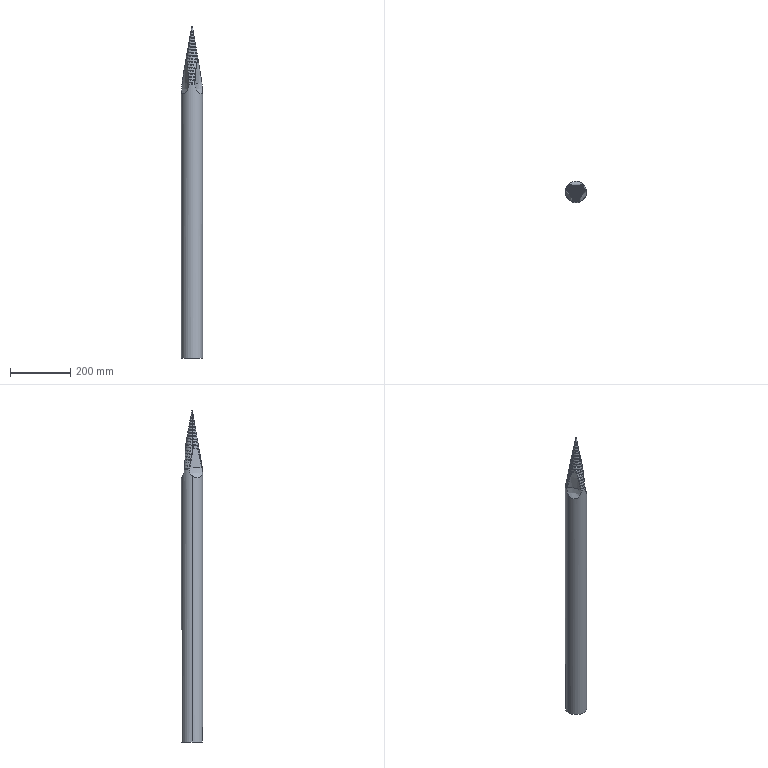Part | SolidWorks | features Chamfer 2, Fillet 2, Cut 1, Extrusion 1, Helix 1, ICE 1, SweepCut 1 | 1 solid | 87 faces | box 70 x 70 x 1100 mm | volume 2879786 mm3 | cone 48 | spline 26 | cylinder 9 | plane 4 | commonest cylinder face diameters 160 x5 50 x2 70 x2